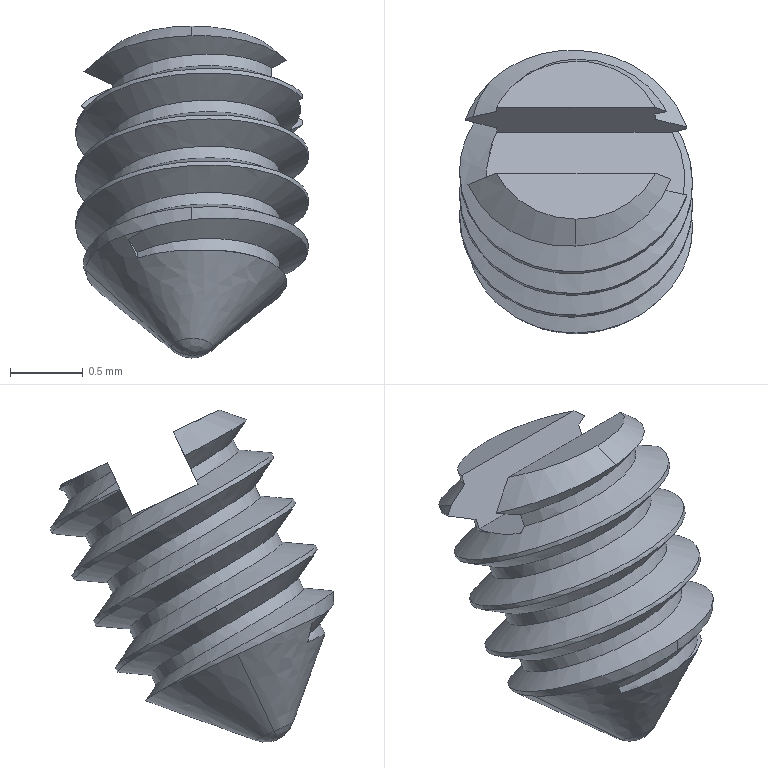Part | SolidWorks | features BaseBody 1 | 1 solid | 34 faces | box 1.6 x 1.946 x 2.281 mm | volume 2.431 mm3 | spline 34